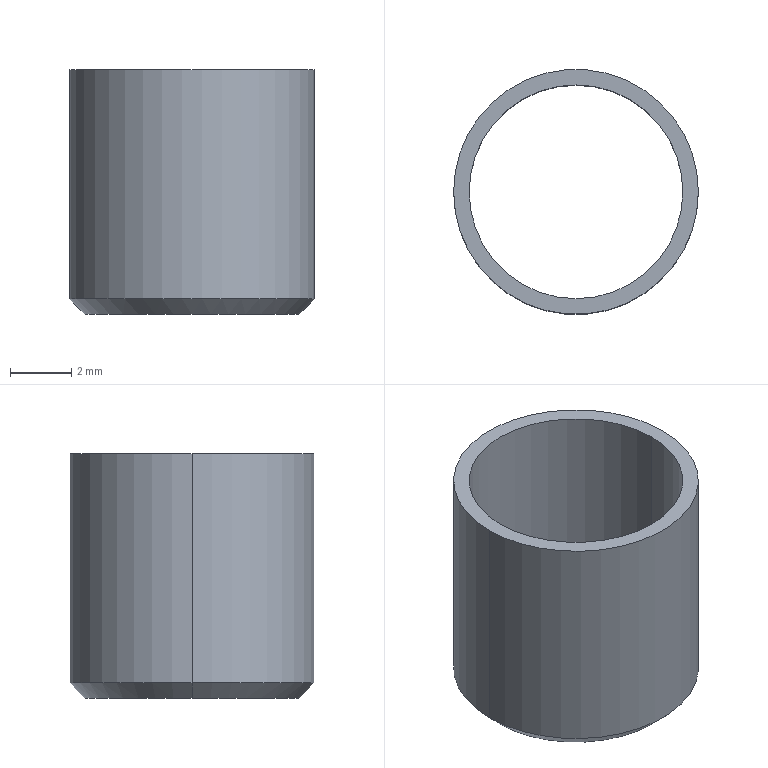Part | Creo | 1 solid | 7 faces | box 8 x 8 x 8 mm | volume 92.458 mm3 | cylinder 4 | cone 2 | plane 1 | commonest cylinder face diameters 6.985 x2 8 x2
STEP:
#1=CARTESIAN_POINT('',(0.,0.,0.));
#2=DIRECTION('',(0.,0.,1.));
#3=DIRECTION('',(1.,0.,0.));
#4=AXIS2_PLACEMENT_3D('',#1,#2,#3);
#5=CARTESIAN_POINT('',(349.386,-109.244,-56.844));
#6=VERTEX_POINT('',#5);
#7=CARTESIAN_POINT('',(341.386,-109.244,-56.844));
#8=VERTEX_POINT('',#7);
#9=CARTESIAN_POINT('',(345.386,-109.244,-56.844));
#10=DIRECTION('',(0.,0.,1.));
#11=DIRECTION('',(1.,0.,0.));
#12=AXIS2_PLACEMENT_3D('',#9,#10,#11);
#13=CIRCLE('',#12,4.);
#14=EDGE_CURVE('',#6,#8,#13,.T.);
#15=ORIENTED_EDGE('',*,*,#14,.T.);
#16=CARTESIAN_POINT('',(341.386,-109.244,-64.336));
#17=VERTEX_POINT('',#16);
#18=CARTESIAN_POINT('',(341.386,-109.244,-56.844));
#19=DIRECTION('',(0.,0.,-1.));
#20=VECTOR('',#19,7.493);
#21=LINE('',#18,#20);
#22=EDGE_CURVE('',#8,#17,#21,.T.);
#23=ORIENTED_EDGE('',*,*,#22,.T.);
#24=CARTESIAN_POINT('',(349.386,-109.244,-64.336));
#25=VERTEX_POINT('',#24);
#26=CARTESIAN_POINT('',(345.386,-109.244,-64.336));
#27=DIRECTION('',(0.,0.,-1.));
#28=DIRECTION('',(-1.,0.,0.));
#29=AXIS2_PLACEMENT_3D('',#26,#27,#28);
#30=CIRCLE('',#29,4.);
#31=EDGE_CURVE('',#17,#25,#30,.T.);
#32=ORIENTED_EDGE('',*,*,#31,.T.);
#33=CARTESIAN_POINT('',(349.386,-109.244,-56.844));
#34=DIRECTION('',(0.,0.,-1.));
#35=VECTOR('',#34,7.493);
#36=LINE('',#33,#35);
#37=EDGE_CURVE('',#6,#25,#36,.T.);
#38=ORIENTED_EDGE('',*,*,#37,.F.);
#39=EDGE_LOOP('',(#15,#23,#32,#38));
#40=FACE_OUTER_BOUND('',#39,.F.);
#41=CARTESIAN_POINT('',(345.386,-109.244,-40.844));
#42=DIRECTION('',(0.,0.,-1.));
#43=DIRECTION('',(-1.,0.,0.));
#44=AXIS2_PLACEMENT_3D('',#41,#42,#43);
#45=CYLINDRICAL_SURFACE('',#44,4.);
#46=ADVANCED_FACE('',(#40),#45,.T.);
#47=ORIENTED_EDGE('',*,*,#14,.F.);
#48=CARTESIAN_POINT('',(345.386,-109.244,-56.844));
#49=DIRECTION('',(0.,0.,1.));
#50=DIRECTION('',(-1.,0.,0.));
#51=AXIS2_PLACEMENT_3D('',#48,#49,#50);
#52=CIRCLE('',#51,4.);
#53=EDGE_CURVE('',#8,#6,#52,.T.);
#54=ORIENTED_EDGE('',*,*,#53,.F.);
#55=EDGE_LOOP('',(#47,#54));
#56=FACE_OUTER_BOUND('',#55,.F.);
#57=CARTESIAN_POINT('',(348.878,-109.244,-56.844));
#58=VERTEX_POINT('',#57);
#59=CARTESIAN_POINT('',(341.893,-109.244,-56.844));
#60=VERTEX_POINT('',#59);
#61=CARTESIAN_POINT('',(345.386,-109.244,-56.844));
#62=DIRECTION('',(0.,0.,-1.));
#63=DIRECTION('',(1.,0.,0.));
#64=AXIS2_PLACEMENT_3D('',#61,#62,#63);
#65=CIRCLE('',#64,3.493);
#66=EDGE_CURVE('',#58,#60,#65,.T.);
#67=ORIENTED_EDGE('',*,*,#66,.F.);
#68=CARTESIAN_POINT('',(345.386,-109.244,-56.844));
#69=DIRECTION('',(0.,0.,-1.));
#70=DIRECTION('',(-1.,0.,0.));
#71=AXIS2_PLACEMENT_3D('',#68,#69,#70);
#72=CIRCLE('',#71,3.493);
#73=EDGE_CURVE('',#60,#58,#72,.T.);
#74=ORIENTED_EDGE('',*,*,#73,.F.);
#75=EDGE_LOOP('',(#67,#74));
#76=FACE_BOUND('',#75,.F.);
#77=CARTESIAN_POINT('',(345.386,-109.244,-56.844));
#78=DIRECTION('',(0.,0.,-1.));
#79=DIRECTION('',(-1.,0.,0.));
#80=AXIS2_PLACEMENT_3D('',#77,#78,#79);
#81=PLANE('',#80);
#82=ADVANCED_FACE('',(#56,#76),#81,.F.);
#83=CARTESIAN_POINT('',(341.893,-109.244,-64.844));
#84=VERTEX_POINT('',#83);
#85=CARTESIAN_POINT('',(348.878,-109.244,-64.844));
#86=VERTEX_POINT('',#85);
#87=CARTESIAN_POINT('',(345.386,-109.244,-64.844));
#88=DIRECTION('',(0.,0.,1.));
#89=DIRECTION('',(-1.,0.,0.));
#90=AXIS2_PLACEMENT_3D('',#87,#88,#89);
#91=CIRCLE('',#90,3.493);
#92=EDGE_CURVE('',#84,#86,#91,.T.);
#93=ORIENTED_EDGE('',*,*,#92,.T.);
#94=CARTESIAN_POINT('',(348.878,-109.244,-56.844));
#95=DIRECTION('',(0.,0.,-1.));
#96=VECTOR('',#95,8.);
#97=LINE('',#94,#96);
#98=EDGE_CURVE('',#58,#86,#97,.T.);
#99=ORIENTED_EDGE('',*,*,#98,.F.);
#100=ORIENTED_EDGE('',*,*,#66,.T.);
#101=CARTESIAN_POINT('',(341.893,-109.244,-56.844));
#102=DIRECTION('',(0.,0.,-1.));
#103=VECTOR('',#102,8.);
#104=LINE('',#101,#103);
#105=EDGE_CURVE('',#60,#84,#104,.T.);
#106=ORIENTED_EDGE('',*,*,#105,.T.);
#107=EDGE_LOOP('',(#93,#99,#100,#106));
#108=FACE_OUTER_BOUND('',#107,.F.);
#109=CARTESIAN_POINT('',(345.386,-109.244,-40.844));
#110=DIRECTION('',(0.,0.,-1.));
#111=DIRECTION('',(-1.,0.,0.));
#112=AXIS2_PLACEMENT_3D('',#109,#110,#111);
#113=CYLINDRICAL_SURFACE('',#112,3.493);
#114=ADVANCED_FACE('',(#108),#113,.F.);
#115=ORIENTED_EDGE('',*,*,#92,.F.);
#116=CARTESIAN_POINT('',(341.893,-109.244,-64.844));
#117=DIRECTION('',(-0.7071,0.,0.7071));
#118=VECTOR('',#117,0.7176);
#119=LINE('',#116,#118);
#120=EDGE_CURVE('',#84,#17,#119,.T.);
#121=ORIENTED_EDGE('',*,*,#120,.T.);
#122=CARTESIAN_POINT('',(345.386,-109.244,-64.336));
#123=DIRECTION('',(0.,0.,-1.));
#124=DIRECTION('',(1.,0.,0.));
#125=AXIS2_PLACEMENT_3D('',#122,#123,#124);
#126=CIRCLE('',#125,4.);
#127=EDGE_CURVE('',#25,#17,#126,.T.);
#128=ORIENTED_EDGE('',*,*,#127,.F.);
#129=CARTESIAN_POINT('',(348.878,-109.244,-64.844));
#130=DIRECTION('',(0.7071,0.,0.7071));
#131=VECTOR('',#130,0.7176);
#132=LINE('',#129,#131);
#133=EDGE_CURVE('',#86,#25,#132,.T.);
#134=ORIENTED_EDGE('',*,*,#133,.F.);
#135=EDGE_LOOP('',(#115,#121,#128,#134));
#136=FACE_OUTER_BOUND('',#135,.F.);
#137=CARTESIAN_POINT('',(345.386,-109.244,-64.59));
#138=DIRECTION('',(0.,0.,1.));
#139=DIRECTION('',(1.,0.,0.));
#140=AXIS2_PLACEMENT_3D('',#137,#138,#139);
#141=CONICAL_SURFACE('',#140,3.746,45.);
#142=ADVANCED_FACE('',(#136),#141,.T.);
#143=CARTESIAN_POINT('',(345.386,-109.244,-64.844));
#144=DIRECTION('',(0.,0.,1.));
#145=DIRECTION('',(1.,0.,0.));
#146=AXIS2_PLACEMENT_3D('',#143,#144,#145);
#147=CIRCLE('',#146,3.493);
#148=EDGE_CURVE('',#86,#84,#147,.T.);
#149=ORIENTED_EDGE('',*,*,#148,.F.);
#150=ORIENTED_EDGE('',*,*,#133,.T.);
#151=ORIENTED_EDGE('',*,*,#31,.F.);
#152=ORIENTED_EDGE('',*,*,#120,.F.);
#153=EDGE_LOOP('',(#149,#150,#151,#152));
#154=FACE_OUTER_BOUND('',#153,.F.);
#155=CARTESIAN_POINT('',(345.386,-109.244,-64.59));
#156=DIRECTION('',(0.,0.,1.));
#157=DIRECTION('',(1.,0.,0.));
#158=AXIS2_PLACEMENT_3D('',#155,#156,#157);
#159=CONICAL_SURFACE('',#158,3.746,45.);
#160=ADVANCED_FACE('',(#154),#159,.T.);
#161=ORIENTED_EDGE('',*,*,#148,.T.);
#162=ORIENTED_EDGE('',*,*,#105,.F.);
#163=ORIENTED_EDGE('',*,*,#73,.T.);
#164=ORIENTED_EDGE('',*,*,#98,.T.);
#165=EDGE_LOOP('',(#161,#162,#163,#164));
#166=FACE_OUTER_BOUND('',#165,.F.);
#167=CARTESIAN_POINT('',(345.386,-109.244,-40.844));
#168=DIRECTION('',(0.,0.,-1.));
#169=DIRECTION('',(-1.,0.,0.));
#170=AXIS2_PLACEMENT_3D('',#167,#168,#169);
#171=CYLINDRICAL_SURFACE('',#170,3.493);
#172=ADVANCED_FACE('',(#166),#171,.F.);
#173=ORIENTED_EDGE('',*,*,#53,.T.);
#174=ORIENTED_EDGE('',*,*,#37,.T.);
#175=ORIENTED_EDGE('',*,*,#127,.T.);
#176=ORIENTED_EDGE('',*,*,#22,.F.);
#177=EDGE_LOOP('',(#173,#174,#175,#176));
#178=FACE_OUTER_BOUND('',#177,.F.);
#179=CARTESIAN_POINT('',(345.386,-109.244,-40.844));
#180=DIRECTION('',(0.,0.,-1.));
#181=DIRECTION('',(-1.,0.,0.));
#182=AXIS2_PLACEMENT_3D('',#179,#180,#181);
#183=CYLINDRICAL_SURFACE('',#182,4.);
#184=ADVANCED_FACE('',(#178),#183,.T.);
#185=CLOSED_SHELL('',(#46,#82,#114,#142,#160,#172,#184));
#186=MANIFOLD_SOLID_BREP('',#185);
#187=(LENGTH_UNIT()NAMED_UNIT(*)SI_UNIT(.MILLI.,.METRE.));
#188=UNCERTAINTY_MEASURE_WITH_UNIT(LENGTH_MEASURE(0.001386),#187,'','');
#189=(NAMED_UNIT(*)PLANE_ANGLE_UNIT()SI_UNIT($,.RADIAN.));
#190=PLANE_ANGLE_MEASURE_WITH_UNIT(PLANE_ANGLE_MEASURE(0.01745),#189);
#191=(CONVERSION_BASED_UNIT('DEGREE',#190)NAMED_UNIT(*)PLANE_ANGLE_UNIT());
#192=(NAMED_UNIT(*)SI_UNIT($,.STERADIAN.)SOLID_ANGLE_UNIT());
#193=(GEOMETRIC_REPRESENTATION_CONTEXT(3)GLOBAL_UNCERTAINTY_ASSIGNED_CONTEXT((#188))GLOBAL_UNIT_ASSIGNED_CONTEXT((#187,#191,#192))REPRESENTATION_CONTEXT('',''));
#194=ADVANCED_BREP_SHAPE_REPRESENTATION('',(#4,#186),#193);